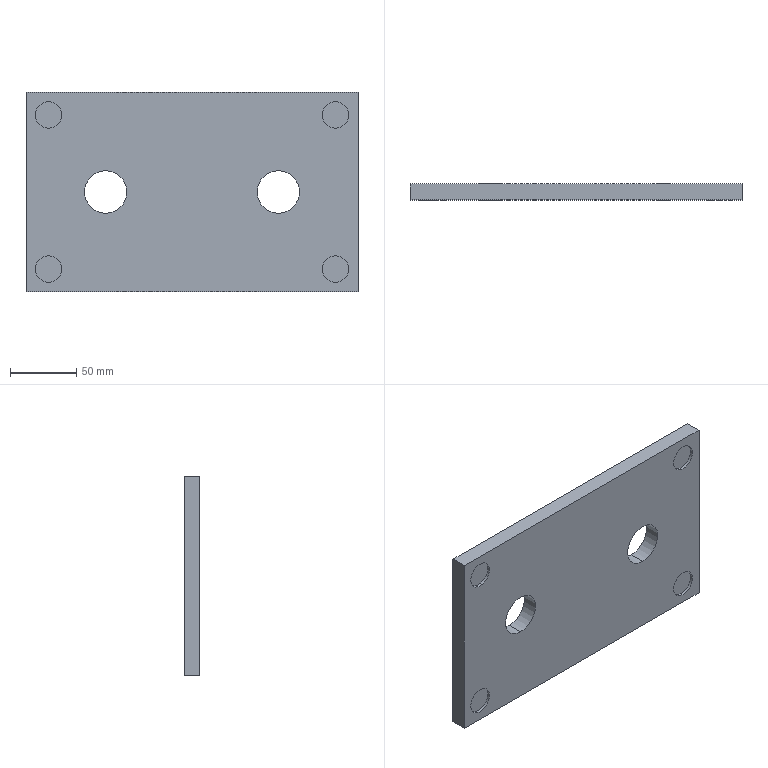Part | SolidWorks | features ICE 2, Extrusion 1 | 1 solid | 22 faces | box 250 x 12 x 150 mm | volume 428185 mm3 | cylinder 12 | plane 10 | commonest cylinder face diameters 20 x8 32 x4
STEP:
#1=CARTESIAN_POINT('',(-65.,0.,-16.));
#2=VERTEX_POINT('',#1);
#3=CARTESIAN_POINT('',(-65.,0.,16.));
#4=VERTEX_POINT('',#3);
#5=CARTESIAN_POINT('',(-65.,0.,0.));
#6=DIRECTION('',(0.,1.,0.));
#7=DIRECTION('',(0.,0.,-1.));
#8=AXIS2_PLACEMENT_3D('',#5,#6,#7);
#9=CIRCLE('',#8,16.);
#10=EDGE_CURVE('',#2,#4,#9,.T.);
#11=ORIENTED_EDGE('',*,*,#10,.F.);
#12=CARTESIAN_POINT('',(-65.,12.,-16.));
#13=VERTEX_POINT('',#12);
#14=CARTESIAN_POINT('',(-65.,-0.001,-16.));
#15=DIRECTION('',(0.,1.,0.));
#16=VECTOR('',#15,1000.);
#17=LINE('',#14,#16);
#18=EDGE_CURVE('',#2,#13,#17,.T.);
#19=ORIENTED_EDGE('',*,*,#18,.T.);
#20=CARTESIAN_POINT('',(-65.,12.,16.));
#21=VERTEX_POINT('',#20);
#22=CARTESIAN_POINT('',(-65.,12.,0.));
#23=DIRECTION('',(0.,1.,0.));
#24=DIRECTION('',(0.,0.,1.));
#25=AXIS2_PLACEMENT_3D('',#22,#23,#24);
#26=CIRCLE('',#25,16.);
#27=EDGE_CURVE('',#13,#21,#26,.T.);
#28=ORIENTED_EDGE('',*,*,#27,.T.);
#29=CARTESIAN_POINT('',(-65.,-0.001,16.));
#30=DIRECTION('',(0.,1.,0.));
#31=VECTOR('',#30,1000.);
#32=LINE('',#29,#31);
#33=EDGE_CURVE('',#4,#21,#32,.T.);
#34=ORIENTED_EDGE('',*,*,#33,.F.);
#35=EDGE_LOOP('',(#11,#19,#28,#34));
#36=FACE_OUTER_BOUND('',#35,.T.);
#37=CARTESIAN_POINT('',(-65.,-0.001,0.));
#38=DIRECTION('',(0.,1.,0.));
#39=DIRECTION('',(0.,0.,1.));
#40=AXIS2_PLACEMENT_3D('',#37,#38,#39);
#41=CYLINDRICAL_SURFACE('',#40,16.);
#42=ADVANCED_FACE('',(#36),#41,.F.);
#43=CARTESIAN_POINT('',(65.,0.,-16.));
#44=VERTEX_POINT('',#43);
#45=CARTESIAN_POINT('',(65.,0.,16.));
#46=VERTEX_POINT('',#45);
#47=CARTESIAN_POINT('',(65.,0.,0.));
#48=DIRECTION('',(0.,1.,0.));
#49=DIRECTION('',(0.,0.,-1.));
#50=AXIS2_PLACEMENT_3D('',#47,#48,#49);
#51=CIRCLE('',#50,16.);
#52=EDGE_CURVE('',#44,#46,#51,.T.);
#53=ORIENTED_EDGE('',*,*,#52,.F.);
#54=CARTESIAN_POINT('',(65.,12.,-16.));
#55=VERTEX_POINT('',#54);
#56=CARTESIAN_POINT('',(65.,-0.001,-16.));
#57=DIRECTION('',(0.,1.,0.));
#58=VECTOR('',#57,1000.);
#59=LINE('',#56,#58);
#60=EDGE_CURVE('',#44,#55,#59,.T.);
#61=ORIENTED_EDGE('',*,*,#60,.T.);
#62=CARTESIAN_POINT('',(65.,12.,16.));
#63=VERTEX_POINT('',#62);
#64=CARTESIAN_POINT('',(65.,12.,0.));
#65=DIRECTION('',(0.,1.,0.));
#66=DIRECTION('',(0.,0.,1.));
#67=AXIS2_PLACEMENT_3D('',#64,#65,#66);
#68=CIRCLE('',#67,16.);
#69=EDGE_CURVE('',#55,#63,#68,.T.);
#70=ORIENTED_EDGE('',*,*,#69,.T.);
#71=CARTESIAN_POINT('',(65.,-0.001,16.));
#72=DIRECTION('',(0.,1.,0.));
#73=VECTOR('',#72,1000.);
#74=LINE('',#71,#73);
#75=EDGE_CURVE('',#46,#63,#74,.T.);
#76=ORIENTED_EDGE('',*,*,#75,.F.);
#77=EDGE_LOOP('',(#53,#61,#70,#76));
#78=FACE_OUTER_BOUND('',#77,.T.);
#79=CARTESIAN_POINT('',(65.,-0.001,0.));
#80=DIRECTION('',(0.,1.,0.));
#81=DIRECTION('',(0.,0.,1.));
#82=AXIS2_PLACEMENT_3D('',#79,#80,#81);
#83=CYLINDRICAL_SURFACE('',#82,16.);
#84=ADVANCED_FACE('',(#78),#83,.F.);
#85=CARTESIAN_POINT('',(-108.,2.,-48.));
#86=VERTEX_POINT('',#85);
#87=CARTESIAN_POINT('',(-108.,2.,-68.));
#88=VERTEX_POINT('',#87);
#89=CARTESIAN_POINT('',(-108.,2.,-58.));
#90=DIRECTION('',(0.,-1.,0.));
#91=DIRECTION('',(0.,0.,-1.));
#92=AXIS2_PLACEMENT_3D('',#89,#90,#91);
#93=CIRCLE('',#92,10.);
#94=EDGE_CURVE('',#86,#88,#93,.T.);
#95=ORIENTED_EDGE('',*,*,#94,.F.);
#96=CARTESIAN_POINT('',(-108.,0.,-48.));
#97=VERTEX_POINT('',#96);
#98=CARTESIAN_POINT('',(-108.,2.,-48.));
#99=DIRECTION('',(0.,-1.,0.));
#100=VECTOR('',#99,1000.);
#101=LINE('',#98,#100);
#102=EDGE_CURVE('',#86,#97,#101,.T.);
#103=ORIENTED_EDGE('',*,*,#102,.T.);
#104=CARTESIAN_POINT('',(-108.,0.,-68.));
#105=VERTEX_POINT('',#104);
#106=CARTESIAN_POINT('',(-108.,0.,-58.));
#107=DIRECTION('',(0.,-1.,0.));
#108=DIRECTION('',(0.,0.,-1.));
#109=AXIS2_PLACEMENT_3D('',#106,#107,#108);
#110=CIRCLE('',#109,10.);
#111=EDGE_CURVE('',#97,#105,#110,.T.);
#112=ORIENTED_EDGE('',*,*,#111,.T.);
#113=CARTESIAN_POINT('',(-108.,2.,-68.));
#114=DIRECTION('',(0.,-1.,0.));
#115=VECTOR('',#114,1000.);
#116=LINE('',#113,#115);
#117=EDGE_CURVE('',#88,#105,#116,.T.);
#118=ORIENTED_EDGE('',*,*,#117,.F.);
#119=EDGE_LOOP('',(#95,#103,#112,#118));
#120=FACE_OUTER_BOUND('',#119,.T.);
#121=CARTESIAN_POINT('',(-108.,2.,-58.));
#122=DIRECTION('',(0.,-1.,0.));
#123=DIRECTION('',(0.,0.,-1.));
#124=AXIS2_PLACEMENT_3D('',#121,#122,#123);
#125=CYLINDRICAL_SURFACE('',#124,10.);
#126=ADVANCED_FACE('',(#120),#125,.F.);
#127=CARTESIAN_POINT('',(108.,2.,68.));
#128=VERTEX_POINT('',#127);
#129=CARTESIAN_POINT('',(108.,2.,48.));
#130=VERTEX_POINT('',#129);
#131=CARTESIAN_POINT('',(108.,2.,58.));
#132=DIRECTION('',(0.,-1.,0.));
#133=DIRECTION('',(0.,0.,-1.));
#134=AXIS2_PLACEMENT_3D('',#131,#132,#133);
#135=CIRCLE('',#134,10.);
#136=EDGE_CURVE('',#128,#130,#135,.T.);
#137=ORIENTED_EDGE('',*,*,#136,.F.);
#138=CARTESIAN_POINT('',(108.,0.,68.));
#139=VERTEX_POINT('',#138);
#140=CARTESIAN_POINT('',(108.,2.,68.));
#141=DIRECTION('',(0.,-1.,0.));
#142=VECTOR('',#141,1000.);
#143=LINE('',#140,#142);
#144=EDGE_CURVE('',#128,#139,#143,.T.);
#145=ORIENTED_EDGE('',*,*,#144,.T.);
#146=CARTESIAN_POINT('',(108.,0.,48.));
#147=VERTEX_POINT('',#146);
#148=CARTESIAN_POINT('',(108.,0.,58.));
#149=DIRECTION('',(0.,-1.,0.));
#150=DIRECTION('',(0.,0.,-1.));
#151=AXIS2_PLACEMENT_3D('',#148,#149,#150);
#152=CIRCLE('',#151,10.);
#153=EDGE_CURVE('',#139,#147,#152,.T.);
#154=ORIENTED_EDGE('',*,*,#153,.T.);
#155=CARTESIAN_POINT('',(108.,2.,48.));
#156=DIRECTION('',(0.,-1.,0.));
#157=VECTOR('',#156,1000.);
#158=LINE('',#155,#157);
#159=EDGE_CURVE('',#130,#147,#158,.T.);
#160=ORIENTED_EDGE('',*,*,#159,.F.);
#161=EDGE_LOOP('',(#137,#145,#154,#160));
#162=FACE_OUTER_BOUND('',#161,.T.);
#163=CARTESIAN_POINT('',(108.,2.,58.));
#164=DIRECTION('',(0.,-1.,0.));
#165=DIRECTION('',(0.,0.,-1.));
#166=AXIS2_PLACEMENT_3D('',#163,#164,#165);
#167=CYLINDRICAL_SURFACE('',#166,10.);
#168=ADVANCED_FACE('',(#162),#167,.F.);
#169=CARTESIAN_POINT('',(-108.,2.,68.));
#170=VERTEX_POINT('',#169);
#171=CARTESIAN_POINT('',(-108.,2.,48.));
#172=VERTEX_POINT('',#171);
#173=CARTESIAN_POINT('',(-108.,2.,58.));
#174=DIRECTION('',(0.,-1.,0.));
#175=DIRECTION('',(0.,0.,-1.));
#176=AXIS2_PLACEMENT_3D('',#173,#174,#175);
#177=CIRCLE('',#176,10.);
#178=EDGE_CURVE('',#170,#172,#177,.T.);
#179=ORIENTED_EDGE('',*,*,#178,.F.);
#180=CARTESIAN_POINT('',(-108.,0.,68.));
#181=VERTEX_POINT('',#180);
#182=CARTESIAN_POINT('',(-108.,2.,68.));
#183=DIRECTION('',(0.,-1.,0.));
#184=VECTOR('',#183,1000.);
#185=LINE('',#182,#184);
#186=EDGE_CURVE('',#170,#181,#185,.T.);
#187=ORIENTED_EDGE('',*,*,#186,.T.);
#188=CARTESIAN_POINT('',(-108.,0.,48.));
#189=VERTEX_POINT('',#188);
#190=CARTESIAN_POINT('',(-108.,0.,58.));
#191=DIRECTION('',(0.,-1.,0.));
#192=DIRECTION('',(0.,0.,-1.));
#193=AXIS2_PLACEMENT_3D('',#190,#191,#192);
#194=CIRCLE('',#193,10.);
#195=EDGE_CURVE('',#181,#189,#194,.T.);
#196=ORIENTED_EDGE('',*,*,#195,.T.);
#197=CARTESIAN_POINT('',(-108.,2.,48.));
#198=DIRECTION('',(0.,-1.,0.));
#199=VECTOR('',#198,1000.);
#200=LINE('',#197,#199);
#201=EDGE_CURVE('',#172,#189,#200,.T.);
#202=ORIENTED_EDGE('',*,*,#201,.F.);
#203=EDGE_LOOP('',(#179,#187,#196,#202));
#204=FACE_OUTER_BOUND('',#203,.T.);
#205=CARTESIAN_POINT('',(-108.,2.,58.));
#206=DIRECTION('',(0.,-1.,0.));
#207=DIRECTION('',(0.,0.,-1.));
#208=AXIS2_PLACEMENT_3D('',#205,#206,#207);
#209=CYLINDRICAL_SURFACE('',#208,10.);
#210=ADVANCED_FACE('',(#204),#209,.F.);
#211=CARTESIAN_POINT('',(108.,2.,-48.));
#212=VERTEX_POINT('',#211);
#213=CARTESIAN_POINT('',(108.,2.,-68.));
#214=VERTEX_POINT('',#213);
#215=CARTESIAN_POINT('',(108.,2.,-58.));
#216=DIRECTION('',(0.,-1.,0.));
#217=DIRECTION('',(0.,0.,-1.));
#218=AXIS2_PLACEMENT_3D('',#215,#216,#217);
#219=CIRCLE('',#218,10.);
#220=EDGE_CURVE('',#212,#214,#219,.T.);
#221=ORIENTED_EDGE('',*,*,#220,.F.);
#222=CARTESIAN_POINT('',(108.,0.,-48.));
#223=VERTEX_POINT('',#222);
#224=CARTESIAN_POINT('',(108.,2.,-48.));
#225=DIRECTION('',(0.,-1.,0.));
#226=VECTOR('',#225,1000.);
#227=LINE('',#224,#226);
#228=EDGE_CURVE('',#212,#223,#227,.T.);
#229=ORIENTED_EDGE('',*,*,#228,.T.);
#230=CARTESIAN_POINT('',(108.,0.,-68.));
#231=VERTEX_POINT('',#230);
#232=CARTESIAN_POINT('',(108.,0.,-58.));
#233=DIRECTION('',(0.,-1.,0.));
#234=DIRECTION('',(0.,0.,-1.));
#235=AXIS2_PLACEMENT_3D('',#232,#233,#234);
#236=CIRCLE('',#235,10.);
#237=EDGE_CURVE('',#223,#231,#236,.T.);
#238=ORIENTED_EDGE('',*,*,#237,.T.);
#239=CARTESIAN_POINT('',(108.,2.,-68.));
#240=DIRECTION('',(0.,-1.,0.));
#241=VECTOR('',#240,1000.);
#242=LINE('',#239,#241);
#243=EDGE_CURVE('',#214,#231,#242,.T.);
#244=ORIENTED_EDGE('',*,*,#243,.F.);
#245=EDGE_LOOP('',(#221,#229,#238,#244));
#246=FACE_OUTER_BOUND('',#245,.T.);
#247=CARTESIAN_POINT('',(108.,2.,-58.));
#248=DIRECTION('',(0.,-1.,0.));
#249=DIRECTION('',(0.,0.,-1.));
#250=AXIS2_PLACEMENT_3D('',#247,#248,#249);
#251=CYLINDRICAL_SURFACE('',#250,10.);
#252=ADVANCED_FACE('',(#246),#251,.F.);
#253=CARTESIAN_POINT('',(125.,0.,75.));
#254=VERTEX_POINT('',#253);
#255=CARTESIAN_POINT('',(125.,0.,-75.));
#256=VERTEX_POINT('',#255);
#257=CARTESIAN_POINT('',(125.,0.,75.));
#258=DIRECTION('',(0.,0.,-1.));
#259=VECTOR('',#258,1000.);
#260=LINE('',#257,#259);
#261=EDGE_CURVE('',#254,#256,#260,.T.);
#262=ORIENTED_EDGE('',*,*,#261,.T.);
#263=CARTESIAN_POINT('',(125.,12.,-75.));
#264=VERTEX_POINT('',#263);
#265=CARTESIAN_POINT('',(125.,12.,-75.));
#266=DIRECTION('',(0.,-1.,0.));
#267=VECTOR('',#266,1000.);
#268=LINE('',#265,#267);
#269=EDGE_CURVE('',#264,#256,#268,.T.);
#270=ORIENTED_EDGE('',*,*,#269,.F.);
#271=CARTESIAN_POINT('',(125.,12.,75.));
#272=VERTEX_POINT('',#271);
#273=CARTESIAN_POINT('',(125.,12.,75.));
#274=DIRECTION('',(0.,0.,-1.));
#275=VECTOR('',#274,1000.);
#276=LINE('',#273,#275);
#277=EDGE_CURVE('',#272,#264,#276,.T.);
#278=ORIENTED_EDGE('',*,*,#277,.F.);
#279=CARTESIAN_POINT('',(125.,12.,75.));
#280=DIRECTION('',(0.,-1.,0.));
#281=VECTOR('',#280,1000.);
#282=LINE('',#279,#281);
#283=EDGE_CURVE('',#272,#254,#282,.T.);
#284=ORIENTED_EDGE('',*,*,#283,.T.);
#285=EDGE_LOOP('',(#262,#270,#278,#284));
#286=FACE_OUTER_BOUND('',#285,.T.);
#287=CARTESIAN_POINT('',(125.,12.,75.));
#288=DIRECTION('',(-1.,0.,0.));
#289=DIRECTION('',(0.,0.,1.));
#290=AXIS2_PLACEMENT_3D('',#287,#288,#289);
#291=PLANE('',#290);
#292=ADVANCED_FACE('',(#286),#291,.F.);
#293=CARTESIAN_POINT('',(-125.,0.,-75.));
#294=VERTEX_POINT('',#293);
#295=CARTESIAN_POINT('',(-125.,0.,-75.));
#296=DIRECTION('',(-1.,0.,0.));
#297=VECTOR('',#296,1000.);
#298=LINE('',#295,#297);
#299=EDGE_CURVE('',#256,#294,#298,.T.);
#300=ORIENTED_EDGE('',*,*,#299,.T.);
#301=CARTESIAN_POINT('',(-125.,12.,-75.));
#302=VERTEX_POINT('',#301);
#303=CARTESIAN_POINT('',(-125.,12.,-75.));
#304=DIRECTION('',(0.,-1.,0.));
#305=VECTOR('',#304,1000.);
#306=LINE('',#303,#305);
#307=EDGE_CURVE('',#302,#294,#306,.T.);
#308=ORIENTED_EDGE('',*,*,#307,.F.);
#309=CARTESIAN_POINT('',(-125.,12.,-75.));
#310=DIRECTION('',(-1.,0.,0.));
#311=VECTOR('',#310,1000.);
#312=LINE('',#309,#311);
#313=EDGE_CURVE('',#264,#302,#312,.T.);
#314=ORIENTED_EDGE('',*,*,#313,.F.);
#315=ORIENTED_EDGE('',*,*,#269,.T.);
#316=EDGE_LOOP('',(#300,#308,#314,#315));
#317=FACE_OUTER_BOUND('',#316,.T.);
#318=CARTESIAN_POINT('',(-125.,12.,-75.));
#319=DIRECTION('',(0.,0.,1.));
#320=DIRECTION('',(1.,0.,0.));
#321=AXIS2_PLACEMENT_3D('',#318,#319,#320);
#322=PLANE('',#321);
#323=ADVANCED_FACE('',(#317),#322,.F.);
#324=CARTESIAN_POINT('',(-125.,0.,75.));
#325=VERTEX_POINT('',#324);
#326=CARTESIAN_POINT('',(-125.,0.,75.));
#327=DIRECTION('',(0.,0.,1.));
#328=VECTOR('',#327,1000.);
#329=LINE('',#326,#328);
#330=EDGE_CURVE('',#294,#325,#329,.T.);
#331=ORIENTED_EDGE('',*,*,#330,.T.);
#332=CARTESIAN_POINT('',(-125.,12.,75.));
#333=VERTEX_POINT('',#332);
#334=CARTESIAN_POINT('',(-125.,12.,75.));
#335=DIRECTION('',(0.,-1.,0.));
#336=VECTOR('',#335,1000.);
#337=LINE('',#334,#336);
#338=EDGE_CURVE('',#333,#325,#337,.T.);
#339=ORIENTED_EDGE('',*,*,#338,.F.);
#340=CARTESIAN_POINT('',(-125.,12.,75.));
#341=DIRECTION('',(0.,0.,1.));
#342=VECTOR('',#341,1000.);
#343=LINE('',#340,#342);
#344=EDGE_CURVE('',#302,#333,#343,.T.);
#345=ORIENTED_EDGE('',*,*,#344,.F.);
#346=ORIENTED_EDGE('',*,*,#307,.T.);
#347=EDGE_LOOP('',(#331,#339,#345,#346));
#348=FACE_OUTER_BOUND('',#347,.T.);
#349=CARTESIAN_POINT('',(-125.,12.,75.));
#350=DIRECTION('',(1.,0.,0.));
#351=DIRECTION('',(0.,0.,-1.));
#352=AXIS2_PLACEMENT_3D('',#349,#350,#351);
#353=PLANE('',#352);
#354=ADVANCED_FACE('',(#348),#353,.F.);
#355=CARTESIAN_POINT('',(-125.,0.,75.));
#356=DIRECTION('',(1.,0.,0.));
#357=VECTOR('',#356,1000.);
#358=LINE('',#355,#357);
#359=EDGE_CURVE('',#325,#254,#358,.T.);
#360=ORIENTED_EDGE('',*,*,#359,.T.);
#361=ORIENTED_EDGE('',*,*,#283,.F.);
#362=CARTESIAN_POINT('',(-125.,12.,75.));
#363=DIRECTION('',(1.,0.,0.));
#364=VECTOR('',#363,1000.);
#365=LINE('',#362,#364);
#366=EDGE_CURVE('',#333,#272,#365,.T.);
#367=ORIENTED_EDGE('',*,*,#366,.F.);
#368=ORIENTED_EDGE('',*,*,#338,.T.);
#369=EDGE_LOOP('',(#360,#361,#367,#368));
#370=FACE_OUTER_BOUND('',#369,.T.);
#371=CARTESIAN_POINT('',(-125.,12.,75.));
#372=DIRECTION('',(0.,0.,-1.));
#373=DIRECTION('',(-1.,0.,0.));
#374=AXIS2_PLACEMENT_3D('',#371,#372,#373);
#375=PLANE('',#374);
#376=ADVANCED_FACE('',(#370),#375,.F.);
#377=CARTESIAN_POINT('',(-65.,12.,0.));
#378=DIRECTION('',(0.,1.,0.));
#379=DIRECTION('',(0.,0.,1.));
#380=AXIS2_PLACEMENT_3D('',#377,#378,#379);
#381=CIRCLE('',#380,16.);
#382=EDGE_CURVE('',#21,#13,#381,.T.);
#383=ORIENTED_EDGE('',*,*,#382,.F.);
#384=ORIENTED_EDGE('',*,*,#27,.F.);
#385=EDGE_LOOP('',(#383,#384));
#386=FACE_BOUND('',#385,.T.);
#387=CARTESIAN_POINT('',(65.,12.,0.));
#388=DIRECTION('',(0.,1.,0.));
#389=DIRECTION('',(0.,0.,1.));
#390=AXIS2_PLACEMENT_3D('',#387,#388,#389);
#391=CIRCLE('',#390,16.);
#392=EDGE_CURVE('',#63,#55,#391,.T.);
#393=ORIENTED_EDGE('',*,*,#392,.F.);
#394=ORIENTED_EDGE('',*,*,#69,.F.);
#395=EDGE_LOOP('',(#393,#394));
#396=FACE_BOUND('',#395,.T.);
#397=ORIENTED_EDGE('',*,*,#277,.T.);
#398=ORIENTED_EDGE('',*,*,#313,.T.);
#399=ORIENTED_EDGE('',*,*,#344,.T.);
#400=ORIENTED_EDGE('',*,*,#366,.T.);
#401=EDGE_LOOP('',(#397,#398,#399,#400));
#402=FACE_OUTER_BOUND('',#401,.T.);
#403=CARTESIAN_POINT('',(0.,12.,0.));
#404=DIRECTION('',(0.,-1.,0.));
#405=DIRECTION('',(0.,0.,-1.));
#406=AXIS2_PLACEMENT_3D('',#403,#404,#405);
#407=PLANE('',#406);
#408=ADVANCED_FACE('',(#386,#396,#402),#407,.F.);
#409=CARTESIAN_POINT('',(-65.,0.,0.));
#410=DIRECTION('',(0.,1.,0.));
#411=DIRECTION('',(0.,0.,-1.));
#412=AXIS2_PLACEMENT_3D('',#409,#410,#411);
#413=CIRCLE('',#412,16.);
#414=EDGE_CURVE('',#4,#2,#413,.T.);
#415=ORIENTED_EDGE('',*,*,#414,.T.);
#416=ORIENTED_EDGE('',*,*,#10,.T.);
#417=EDGE_LOOP('',(#415,#416));
#418=FACE_BOUND('',#417,.T.);
#419=CARTESIAN_POINT('',(65.,0.,0.));
#420=DIRECTION('',(0.,1.,0.));
#421=DIRECTION('',(0.,0.,-1.));
#422=AXIS2_PLACEMENT_3D('',#419,#420,#421);
#423=CIRCLE('',#422,16.);
#424=EDGE_CURVE('',#46,#44,#423,.T.);
#425=ORIENTED_EDGE('',*,*,#424,.T.);
#426=ORIENTED_EDGE('',*,*,#52,.T.);
#427=EDGE_LOOP('',(#425,#426));
#428=FACE_BOUND('',#427,.T.);
#429=CARTESIAN_POINT('',(-108.,0.,-58.));
#430=DIRECTION('',(0.,-1.,0.));
#431=DIRECTION('',(0.,0.,-1.));
#432=AXIS2_PLACEMENT_3D('',#429,#430,#431);
#433=CIRCLE('',#432,10.);
#434=EDGE_CURVE('',#105,#97,#433,.T.);
#435=ORIENTED_EDGE('',*,*,#434,.F.);
#436=ORIENTED_EDGE('',*,*,#111,.F.);
#437=EDGE_LOOP('',(#435,#436));
#438=FACE_BOUND('',#437,.T.);
#439=CARTESIAN_POINT('',(108.,0.,58.));
#440=DIRECTION('',(0.,-1.,0.));
#441=DIRECTION('',(0.,0.,-1.));
#442=AXIS2_PLACEMENT_3D('',#439,#440,#441);
#443=CIRCLE('',#442,10.);
#444=EDGE_CURVE('',#147,#139,#443,.T.);
#445=ORIENTED_EDGE('',*,*,#444,.F.);
#446=ORIENTED_EDGE('',*,*,#153,.F.);
#447=EDGE_LOOP('',(#445,#446));
#448=FACE_BOUND('',#447,.T.);
#449=CARTESIAN_POINT('',(-108.,0.,58.));
#450=DIRECTION('',(0.,-1.,0.));
#451=DIRECTION('',(0.,0.,-1.));
#452=AXIS2_PLACEMENT_3D('',#449,#450,#451);
#453=CIRCLE('',#452,10.);
#454=EDGE_CURVE('',#189,#181,#453,.T.);
#455=ORIENTED_EDGE('',*,*,#454,.F.);
#456=ORIENTED_EDGE('',*,*,#195,.F.);
#457=EDGE_LOOP('',(#455,#456));
#458=FACE_BOUND('',#457,.T.);
#459=CARTESIAN_POINT('',(108.,0.,-58.));
#460=DIRECTION('',(0.,-1.,0.));
#461=DIRECTION('',(0.,0.,-1.));
#462=AXIS2_PLACEMENT_3D('',#459,#460,#461);
#463=CIRCLE('',#462,10.);
#464=EDGE_CURVE('',#231,#223,#463,.T.);
#465=ORIENTED_EDGE('',*,*,#464,.F.);
#466=ORIENTED_EDGE('',*,*,#237,.F.);
#467=EDGE_LOOP('',(#465,#466));
#468=FACE_BOUND('',#467,.T.);
#469=ORIENTED_EDGE('',*,*,#261,.F.);
#470=ORIENTED_EDGE('',*,*,#359,.F.);
#471=ORIENTED_EDGE('',*,*,#330,.F.);
#472=ORIENTED_EDGE('',*,*,#299,.F.);
#473=EDGE_LOOP('',(#469,#470,#471,#472));
#474=FACE_OUTER_BOUND('',#473,.T.);
#475=CARTESIAN_POINT('',(0.,0.,0.));
#476=DIRECTION('',(0.,-1.,0.));
#477=DIRECTION('',(0.,0.,-1.));
#478=AXIS2_PLACEMENT_3D('',#475,#476,#477);
#479=PLANE('',#478);
#480=ADVANCED_FACE('',(#418,#428,#438,#448,#458,#468,#474),#479,.T.);
#481=ORIENTED_EDGE('',*,*,#228,.F.);
#482=CARTESIAN_POINT('',(108.,2.,-58.));
#483=DIRECTION('',(0.,-1.,0.));
#484=DIRECTION('',(0.,0.,-1.));
#485=AXIS2_PLACEMENT_3D('',#482,#483,#484);
#486=CIRCLE('',#485,10.);
#487=EDGE_CURVE('',#214,#212,#486,.T.);
#488=ORIENTED_EDGE('',*,*,#487,.F.);
#489=ORIENTED_EDGE('',*,*,#243,.T.);
#490=ORIENTED_EDGE('',*,*,#464,.T.);
#491=EDGE_LOOP('',(#481,#488,#489,#490));
#492=FACE_OUTER_BOUND('',#491,.T.);
#493=CARTESIAN_POINT('',(108.,2.,-58.));
#494=DIRECTION('',(0.,-1.,0.));
#495=DIRECTION('',(0.,0.,-1.));
#496=AXIS2_PLACEMENT_3D('',#493,#494,#495);
#497=CYLINDRICAL_SURFACE('',#496,10.);
#498=ADVANCED_FACE('',(#492),#497,.F.);
#499=ORIENTED_EDGE('',*,*,#487,.T.);
#500=ORIENTED_EDGE('',*,*,#220,.T.);
#501=EDGE_LOOP('',(#499,#500));
#502=FACE_OUTER_BOUND('',#501,.T.);
#503=CARTESIAN_POINT('',(108.,2.,-58.));
#504=DIRECTION('',(0.,-1.,0.));
#505=DIRECTION('',(0.,0.,-1.));
#506=AXIS2_PLACEMENT_3D('',#503,#504,#505);
#507=PLANE('',#506);
#508=ADVANCED_FACE('',(#502),#507,.T.);
#509=ORIENTED_EDGE('',*,*,#186,.F.);
#510=CARTESIAN_POINT('',(-108.,2.,58.));
#511=DIRECTION('',(0.,-1.,0.));
#512=DIRECTION('',(0.,0.,-1.));
#513=AXIS2_PLACEMENT_3D('',#510,#511,#512);
#514=CIRCLE('',#513,10.);
#515=EDGE_CURVE('',#172,#170,#514,.T.);
#516=ORIENTED_EDGE('',*,*,#515,.F.);
#517=ORIENTED_EDGE('',*,*,#201,.T.);
#518=ORIENTED_EDGE('',*,*,#454,.T.);
#519=EDGE_LOOP('',(#509,#516,#517,#518));
#520=FACE_OUTER_BOUND('',#519,.T.);
#521=CARTESIAN_POINT('',(-108.,2.,58.));
#522=DIRECTION('',(0.,-1.,0.));
#523=DIRECTION('',(0.,0.,-1.));
#524=AXIS2_PLACEMENT_3D('',#521,#522,#523);
#525=CYLINDRICAL_SURFACE('',#524,10.);
#526=ADVANCED_FACE('',(#520),#525,.F.);
#527=ORIENTED_EDGE('',*,*,#515,.T.);
#528=ORIENTED_EDGE('',*,*,#178,.T.);
#529=EDGE_LOOP('',(#527,#528));
#530=FACE_OUTER_BOUND('',#529,.T.);
#531=CARTESIAN_POINT('',(-108.,2.,58.));
#532=DIRECTION('',(0.,-1.,0.));
#533=DIRECTION('',(0.,0.,-1.));
#534=AXIS2_PLACEMENT_3D('',#531,#532,#533);
#535=PLANE('',#534);
#536=ADVANCED_FACE('',(#530),#535,.T.);
#537=ORIENTED_EDGE('',*,*,#144,.F.);
#538=CARTESIAN_POINT('',(108.,2.,58.));
#539=DIRECTION('',(0.,-1.,0.));
#540=DIRECTION('',(0.,0.,-1.));
#541=AXIS2_PLACEMENT_3D('',#538,#539,#540);
#542=CIRCLE('',#541,10.);
#543=EDGE_CURVE('',#130,#128,#542,.T.);
#544=ORIENTED_EDGE('',*,*,#543,.F.);
#545=ORIENTED_EDGE('',*,*,#159,.T.);
#546=ORIENTED_EDGE('',*,*,#444,.T.);
#547=EDGE_LOOP('',(#537,#544,#545,#546));
#548=FACE_OUTER_BOUND('',#547,.T.);
#549=CARTESIAN_POINT('',(108.,2.,58.));
#550=DIRECTION('',(0.,-1.,0.));
#551=DIRECTION('',(0.,0.,-1.));
#552=AXIS2_PLACEMENT_3D('',#549,#550,#551);
#553=CYLINDRICAL_SURFACE('',#552,10.);
#554=ADVANCED_FACE('',(#548),#553,.F.);
#555=ORIENTED_EDGE('',*,*,#543,.T.);
#556=ORIENTED_EDGE('',*,*,#136,.T.);
#557=EDGE_LOOP('',(#555,#556));
#558=FACE_OUTER_BOUND('',#557,.T.);
#559=CARTESIAN_POINT('',(108.,2.,58.));
#560=DIRECTION('',(0.,-1.,0.));
#561=DIRECTION('',(0.,0.,-1.));
#562=AXIS2_PLACEMENT_3D('',#559,#560,#561);
#563=PLANE('',#562);
#564=ADVANCED_FACE('',(#558),#563,.T.);
#565=ORIENTED_EDGE('',*,*,#102,.F.);
#566=CARTESIAN_POINT('',(-108.,2.,-58.));
#567=DIRECTION('',(0.,-1.,0.));
#568=DIRECTION('',(0.,0.,-1.));
#569=AXIS2_PLACEMENT_3D('',#566,#567,#568);
#570=CIRCLE('',#569,10.);
#571=EDGE_CURVE('',#88,#86,#570,.T.);
#572=ORIENTED_EDGE('',*,*,#571,.F.);
#573=ORIENTED_EDGE('',*,*,#117,.T.);
#574=ORIENTED_EDGE('',*,*,#434,.T.);
#575=EDGE_LOOP('',(#565,#572,#573,#574));
#576=FACE_OUTER_BOUND('',#575,.T.);
#577=CARTESIAN_POINT('',(-108.,2.,-58.));
#578=DIRECTION('',(0.,-1.,0.));
#579=DIRECTION('',(0.,0.,-1.));
#580=AXIS2_PLACEMENT_3D('',#577,#578,#579);
#581=CYLINDRICAL_SURFACE('',#580,10.);
#582=ADVANCED_FACE('',(#576),#581,.F.);
#583=ORIENTED_EDGE('',*,*,#571,.T.);
#584=ORIENTED_EDGE('',*,*,#94,.T.);
#585=EDGE_LOOP('',(#583,#584));
#586=FACE_OUTER_BOUND('',#585,.T.);
#587=CARTESIAN_POINT('',(-108.,2.,-58.));
#588=DIRECTION('',(0.,-1.,0.));
#589=DIRECTION('',(0.,0.,-1.));
#590=AXIS2_PLACEMENT_3D('',#587,#588,#589);
#591=PLANE('',#590);
#592=ADVANCED_FACE('',(#586),#591,.T.);
#593=ORIENTED_EDGE('',*,*,#60,.F.);
#594=ORIENTED_EDGE('',*,*,#424,.F.);
#595=ORIENTED_EDGE('',*,*,#75,.T.);
#596=ORIENTED_EDGE('',*,*,#392,.T.);
#597=EDGE_LOOP('',(#593,#594,#595,#596));
#598=FACE_OUTER_BOUND('',#597,.T.);
#599=CARTESIAN_POINT('',(65.,-0.001,0.));
#600=DIRECTION('',(0.,1.,0.));
#601=DIRECTION('',(0.,0.,1.));
#602=AXIS2_PLACEMENT_3D('',#599,#600,#601);
#603=CYLINDRICAL_SURFACE('',#602,16.);
#604=ADVANCED_FACE('',(#598),#603,.F.);
#605=ORIENTED_EDGE('',*,*,#18,.F.);
#606=ORIENTED_EDGE('',*,*,#414,.F.);
#607=ORIENTED_EDGE('',*,*,#33,.T.);
#608=ORIENTED_EDGE('',*,*,#382,.T.);
#609=EDGE_LOOP('',(#605,#606,#607,#608));
#610=FACE_OUTER_BOUND('',#609,.T.);
#611=CARTESIAN_POINT('',(-65.,-0.001,0.));
#612=DIRECTION('',(0.,1.,0.));
#613=DIRECTION('',(0.,0.,1.));
#614=AXIS2_PLACEMENT_3D('',#611,#612,#613);
#615=CYLINDRICAL_SURFACE('',#614,16.);
#616=ADVANCED_FACE('',(#610),#615,.F.);
#617=CLOSED_SHELL('',(#42,#84,#126,#168,#210,#252,#292,#323,#354,#376,#408,#480,#498,#508,#526,#536,#554,#564,#582,#592,#604,#616));
#618=MANIFOLD_SOLID_BREP('',#617);
#619=CARTESIAN_POINT('',(0.,0.,0.));
#620=DIRECTION('',(0.,0.,1.));
#621=DIRECTION('',(1.,0.,0.));
#622=AXIS2_PLACEMENT_3D('',#619,#620,#621);
#623=(LENGTH_UNIT()NAMED_UNIT(*)SI_UNIT(.MILLI.,.METRE.));
#624=UNCERTAINTY_MEASURE_WITH_UNIT(LENGTH_MEASURE(0.00001),#623,'','');
#625=(NAMED_UNIT(*)PLANE_ANGLE_UNIT()SI_UNIT($,.RADIAN.));
#626=(NAMED_UNIT(*)SI_UNIT($,.STERADIAN.)SOLID_ANGLE_UNIT());
#627=(GEOMETRIC_REPRESENTATION_CONTEXT(3)GLOBAL_UNCERTAINTY_ASSIGNED_CONTEXT((#624))GLOBAL_UNIT_ASSIGNED_CONTEXT((#623,#625,#626))REPRESENTATION_CONTEXT('',''));
#628=ADVANCED_BREP_SHAPE_REPRESENTATION('',(#618,#622),#627);